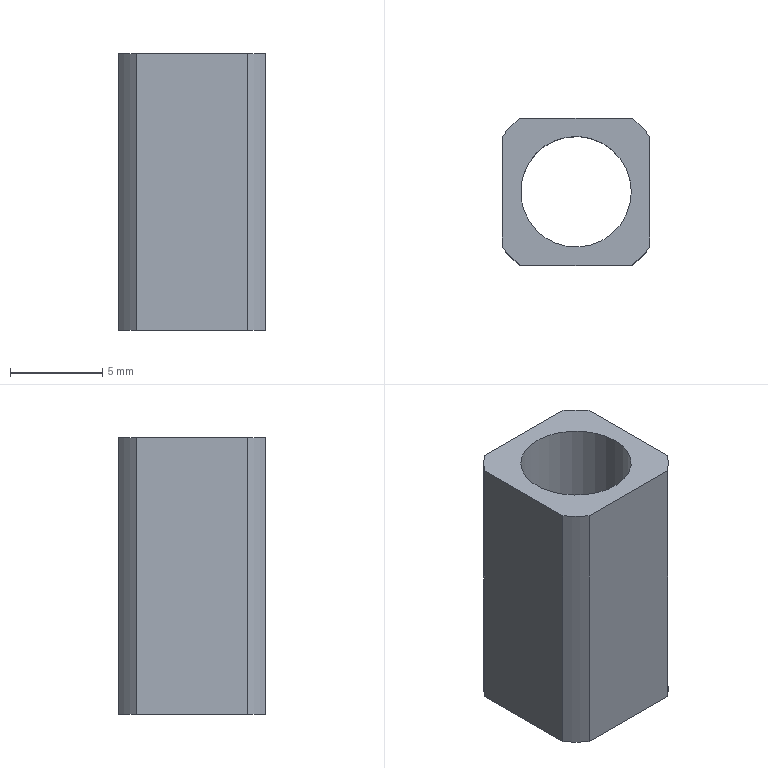Part | NX | 1 solid | 13 faces | box 8 x 8 x 15 mm | volume 464.552 mm3 | plane 7 | cylinder 6 | commonest cylinder face diameters 10 x4 6 x1 6.5 x1
STEP:
#1=CARTESIAN_POINT('',(3.,4.,15.));
#2=VERTEX_POINT('',#1);
#3=CARTESIAN_POINT('',(4.,3.,15.));
#4=VERTEX_POINT('',#3);
#5=CARTESIAN_POINT('',(0.,0.,15.));
#6=DIRECTION('',(0.,0.,-1.));
#7=DIRECTION('',(1.,0.,0.));
#8=AXIS2_PLACEMENT_3D('',#5,#6,#7);
#9=CIRCLE('',#8,5.);
#10=EDGE_CURVE('',#2,#4,#9,.T.);
#11=ORIENTED_EDGE('',*,*,#10,.T.);
#12=CARTESIAN_POINT('',(4.,3.,0.));
#13=VERTEX_POINT('',#12);
#14=CARTESIAN_POINT('',(4.,3.,0.));
#15=DIRECTION('',(0.,0.,1.));
#16=VECTOR('',#15,1000.);
#17=LINE('',#14,#16);
#18=EDGE_CURVE('',#13,#4,#17,.T.);
#19=ORIENTED_EDGE('',*,*,#18,.F.);
#20=CARTESIAN_POINT('',(3.,4.,0.));
#21=VERTEX_POINT('',#20);
#22=CARTESIAN_POINT('',(0.,0.,0.));
#23=DIRECTION('',(0.,0.,1.));
#24=DIRECTION('',(1.,0.,0.));
#25=AXIS2_PLACEMENT_3D('',#22,#23,#24);
#26=CIRCLE('',#25,5.);
#27=EDGE_CURVE('',#13,#21,#26,.T.);
#28=ORIENTED_EDGE('',*,*,#27,.T.);
#29=CARTESIAN_POINT('',(3.,4.,0.));
#30=DIRECTION('',(0.,0.,1.));
#31=VECTOR('',#30,1000.);
#32=LINE('',#29,#31);
#33=EDGE_CURVE('',#21,#2,#32,.T.);
#34=ORIENTED_EDGE('',*,*,#33,.T.);
#35=EDGE_LOOP('',(#11,#19,#28,#34));
#36=FACE_BOUND('',#35,.T.);
#37=CARTESIAN_POINT('',(0.,0.,0.));
#38=DIRECTION('',(0.,0.,1.));
#39=DIRECTION('',(1.,0.,0.));
#40=AXIS2_PLACEMENT_3D('',#37,#38,#39);
#41=CYLINDRICAL_SURFACE('',#40,5.);
#42=ADVANCED_FACE('',(#36),#41,.T.);
#43=CARTESIAN_POINT('',(-3.,4.,0.));
#44=VERTEX_POINT('',#43);
#45=CARTESIAN_POINT('',(-4.,3.,0.));
#46=VERTEX_POINT('',#45);
#47=CARTESIAN_POINT('',(0.,0.,0.));
#48=DIRECTION('',(0.,0.,1.));
#49=DIRECTION('',(1.,0.,0.));
#50=AXIS2_PLACEMENT_3D('',#47,#48,#49);
#51=CIRCLE('',#50,5.);
#52=EDGE_CURVE('',#44,#46,#51,.T.);
#53=ORIENTED_EDGE('',*,*,#52,.T.);
#54=CARTESIAN_POINT('',(-4.,3.,15.));
#55=VERTEX_POINT('',#54);
#56=CARTESIAN_POINT('',(-4.,3.,0.));
#57=DIRECTION('',(0.,0.,1.));
#58=VECTOR('',#57,1000.);
#59=LINE('',#56,#58);
#60=EDGE_CURVE('',#46,#55,#59,.T.);
#61=ORIENTED_EDGE('',*,*,#60,.T.);
#62=CARTESIAN_POINT('',(-3.,4.,15.));
#63=VERTEX_POINT('',#62);
#64=CARTESIAN_POINT('',(0.,0.,15.));
#65=DIRECTION('',(0.,0.,-1.));
#66=DIRECTION('',(1.,0.,0.));
#67=AXIS2_PLACEMENT_3D('',#64,#65,#66);
#68=CIRCLE('',#67,5.);
#69=EDGE_CURVE('',#55,#63,#68,.T.);
#70=ORIENTED_EDGE('',*,*,#69,.T.);
#71=CARTESIAN_POINT('',(-3.,4.,0.));
#72=DIRECTION('',(0.,0.,1.));
#73=VECTOR('',#72,1000.);
#74=LINE('',#71,#73);
#75=EDGE_CURVE('',#63,#44,#74,.F.);
#76=ORIENTED_EDGE('',*,*,#75,.T.);
#77=EDGE_LOOP('',(#53,#61,#70,#76));
#78=FACE_BOUND('',#77,.T.);
#79=CARTESIAN_POINT('',(0.,0.,0.));
#80=DIRECTION('',(0.,0.,1.));
#81=DIRECTION('',(1.,0.,0.));
#82=AXIS2_PLACEMENT_3D('',#79,#80,#81);
#83=CYLINDRICAL_SURFACE('',#82,5.);
#84=ADVANCED_FACE('',(#78),#83,.T.);
#85=CARTESIAN_POINT('',(-4.,-3.,0.));
#86=VERTEX_POINT('',#85);
#87=CARTESIAN_POINT('',(-3.,-4.,0.));
#88=VERTEX_POINT('',#87);
#89=CARTESIAN_POINT('',(0.,0.,0.));
#90=DIRECTION('',(0.,0.,1.));
#91=DIRECTION('',(1.,0.,0.));
#92=AXIS2_PLACEMENT_3D('',#89,#90,#91);
#93=CIRCLE('',#92,5.);
#94=EDGE_CURVE('',#86,#88,#93,.T.);
#95=ORIENTED_EDGE('',*,*,#94,.T.);
#96=CARTESIAN_POINT('',(-3.,-4.,15.));
#97=VERTEX_POINT('',#96);
#98=CARTESIAN_POINT('',(-3.,-4.,0.));
#99=DIRECTION('',(0.,0.,1.));
#100=VECTOR('',#99,1000.);
#101=LINE('',#98,#100);
#102=EDGE_CURVE('',#97,#88,#101,.F.);
#103=ORIENTED_EDGE('',*,*,#102,.F.);
#104=CARTESIAN_POINT('',(-4.,-3.,15.));
#105=VERTEX_POINT('',#104);
#106=CARTESIAN_POINT('',(0.,0.,15.));
#107=DIRECTION('',(0.,0.,-1.));
#108=DIRECTION('',(1.,0.,0.));
#109=AXIS2_PLACEMENT_3D('',#106,#107,#108);
#110=CIRCLE('',#109,5.);
#111=EDGE_CURVE('',#97,#105,#110,.T.);
#112=ORIENTED_EDGE('',*,*,#111,.T.);
#113=CARTESIAN_POINT('',(-4.,-3.,0.));
#114=DIRECTION('',(0.,0.,1.));
#115=VECTOR('',#114,1000.);
#116=LINE('',#113,#115);
#117=EDGE_CURVE('',#105,#86,#116,.F.);
#118=ORIENTED_EDGE('',*,*,#117,.T.);
#119=EDGE_LOOP('',(#95,#103,#112,#118));
#120=FACE_BOUND('',#119,.T.);
#121=CARTESIAN_POINT('',(0.,0.,0.));
#122=DIRECTION('',(0.,0.,1.));
#123=DIRECTION('',(1.,0.,0.));
#124=AXIS2_PLACEMENT_3D('',#121,#122,#123);
#125=CYLINDRICAL_SURFACE('',#124,5.);
#126=ADVANCED_FACE('',(#120),#125,.T.);
#127=CARTESIAN_POINT('',(4.,-3.,15.));
#128=VERTEX_POINT('',#127);
#129=CARTESIAN_POINT('',(3.,-4.,15.));
#130=VERTEX_POINT('',#129);
#131=CARTESIAN_POINT('',(0.,0.,15.));
#132=DIRECTION('',(0.,0.,-1.));
#133=DIRECTION('',(1.,0.,0.));
#134=AXIS2_PLACEMENT_3D('',#131,#132,#133);
#135=CIRCLE('',#134,5.);
#136=EDGE_CURVE('',#128,#130,#135,.T.);
#137=ORIENTED_EDGE('',*,*,#136,.T.);
#138=CARTESIAN_POINT('',(3.,-4.,0.));
#139=VERTEX_POINT('',#138);
#140=CARTESIAN_POINT('',(3.,-4.,0.));
#141=DIRECTION('',(0.,0.,1.));
#142=VECTOR('',#141,1000.);
#143=LINE('',#140,#142);
#144=EDGE_CURVE('',#139,#130,#143,.T.);
#145=ORIENTED_EDGE('',*,*,#144,.F.);
#146=CARTESIAN_POINT('',(4.,-3.,0.));
#147=VERTEX_POINT('',#146);
#148=CARTESIAN_POINT('',(0.,0.,0.));
#149=DIRECTION('',(0.,0.,1.));
#150=DIRECTION('',(1.,0.,0.));
#151=AXIS2_PLACEMENT_3D('',#148,#149,#150);
#152=CIRCLE('',#151,5.);
#153=EDGE_CURVE('',#139,#147,#152,.T.);
#154=ORIENTED_EDGE('',*,*,#153,.T.);
#155=CARTESIAN_POINT('',(4.,-3.,0.));
#156=DIRECTION('',(0.,0.,1.));
#157=VECTOR('',#156,1000.);
#158=LINE('',#155,#157);
#159=EDGE_CURVE('',#128,#147,#158,.F.);
#160=ORIENTED_EDGE('',*,*,#159,.F.);
#161=EDGE_LOOP('',(#137,#145,#154,#160));
#162=FACE_BOUND('',#161,.T.);
#163=CARTESIAN_POINT('',(0.,0.,0.));
#164=DIRECTION('',(0.,0.,1.));
#165=DIRECTION('',(1.,0.,0.));
#166=AXIS2_PLACEMENT_3D('',#163,#164,#165);
#167=CYLINDRICAL_SURFACE('',#166,5.);
#168=ADVANCED_FACE('',(#162),#167,.T.);
#169=CARTESIAN_POINT('',(3.25,0.,0.));
#170=VERTEX_POINT('',#169);
#171=CARTESIAN_POINT('',(0.,0.,0.));
#172=DIRECTION('',(0.,0.,1.));
#173=DIRECTION('',(1.,0.,0.));
#174=AXIS2_PLACEMENT_3D('',#171,#172,#173);
#175=CIRCLE('',#174,3.25);
#176=EDGE_CURVE('',#170,#170,#175,.T.);
#177=ORIENTED_EDGE('',*,*,#176,.T.);
#178=EDGE_LOOP('',(#177));
#179=FACE_BOUND('',#178,.T.);
#180=CARTESIAN_POINT('',(4.,0.,0.));
#181=DIRECTION('',(0.,1.,0.));
#182=VECTOR('',#181,1000.);
#183=LINE('',#180,#182);
#184=EDGE_CURVE('',#13,#147,#183,.F.);
#185=ORIENTED_EDGE('',*,*,#184,.T.);
#186=ORIENTED_EDGE('',*,*,#153,.F.);
#187=CARTESIAN_POINT('',(0.,-4.,0.));
#188=DIRECTION('',(1.,0.,0.));
#189=VECTOR('',#188,1000.);
#190=LINE('',#187,#189);
#191=EDGE_CURVE('',#139,#88,#190,.F.);
#192=ORIENTED_EDGE('',*,*,#191,.T.);
#193=ORIENTED_EDGE('',*,*,#94,.F.);
#194=CARTESIAN_POINT('',(-4.,0.,0.));
#195=DIRECTION('',(0.,-1.,0.));
#196=VECTOR('',#195,1000.);
#197=LINE('',#194,#196);
#198=EDGE_CURVE('',#46,#86,#197,.T.);
#199=ORIENTED_EDGE('',*,*,#198,.F.);
#200=ORIENTED_EDGE('',*,*,#52,.F.);
#201=CARTESIAN_POINT('',(0.,4.,0.));
#202=DIRECTION('',(-1.,0.,0.));
#203=VECTOR('',#202,1000.);
#204=LINE('',#201,#203);
#205=EDGE_CURVE('',#44,#21,#204,.F.);
#206=ORIENTED_EDGE('',*,*,#205,.T.);
#207=ORIENTED_EDGE('',*,*,#27,.F.);
#208=EDGE_LOOP('',(#185,#186,#192,#193,#199,#200,#206,#207));
#209=FACE_BOUND('',#208,.T.);
#210=CARTESIAN_POINT('',(0.,0.,0.));
#211=DIRECTION('',(0.,0.,-1.));
#212=DIRECTION('',(-1.,0.,0.));
#213=AXIS2_PLACEMENT_3D('',#210,#211,#212);
#214=PLANE('',#213);
#215=ADVANCED_FACE('',(#179,#209),#214,.T.);
#216=CARTESIAN_POINT('',(3.,0.,15.));
#217=VERTEX_POINT('',#216);
#218=CARTESIAN_POINT('',(0.,0.,15.));
#219=DIRECTION('',(0.,0.,-1.));
#220=DIRECTION('',(1.,0.,0.));
#221=AXIS2_PLACEMENT_3D('',#218,#219,#220);
#222=CIRCLE('',#221,3.);
#223=EDGE_CURVE('',#217,#217,#222,.T.);
#224=ORIENTED_EDGE('',*,*,#223,.T.);
#225=EDGE_LOOP('',(#224));
#226=FACE_BOUND('',#225,.T.);
#227=CARTESIAN_POINT('',(0.,-4.,15.));
#228=DIRECTION('',(-1.,0.,0.));
#229=VECTOR('',#228,1000.);
#230=LINE('',#227,#229);
#231=EDGE_CURVE('',#130,#97,#230,.T.);
#232=ORIENTED_EDGE('',*,*,#231,.F.);
#233=ORIENTED_EDGE('',*,*,#136,.F.);
#234=CARTESIAN_POINT('',(4.,0.,15.));
#235=DIRECTION('',(0.,-1.,0.));
#236=VECTOR('',#235,1000.);
#237=LINE('',#234,#236);
#238=EDGE_CURVE('',#4,#128,#237,.T.);
#239=ORIENTED_EDGE('',*,*,#238,.F.);
#240=ORIENTED_EDGE('',*,*,#10,.F.);
#241=CARTESIAN_POINT('',(0.,4.,15.));
#242=DIRECTION('',(1.,0.,0.));
#243=VECTOR('',#242,1000.);
#244=LINE('',#241,#243);
#245=EDGE_CURVE('',#63,#2,#244,.T.);
#246=ORIENTED_EDGE('',*,*,#245,.F.);
#247=ORIENTED_EDGE('',*,*,#69,.F.);
#248=CARTESIAN_POINT('',(-4.,0.,15.));
#249=DIRECTION('',(0.,1.,0.));
#250=VECTOR('',#249,1000.);
#251=LINE('',#248,#250);
#252=EDGE_CURVE('',#105,#55,#251,.T.);
#253=ORIENTED_EDGE('',*,*,#252,.F.);
#254=ORIENTED_EDGE('',*,*,#111,.F.);
#255=EDGE_LOOP('',(#232,#233,#239,#240,#246,#247,#253,#254));
#256=FACE_BOUND('',#255,.T.);
#257=CARTESIAN_POINT('',(0.,0.,15.));
#258=DIRECTION('',(0.,0.,1.));
#259=DIRECTION('',(1.,0.,0.));
#260=AXIS2_PLACEMENT_3D('',#257,#258,#259);
#261=PLANE('',#260);
#262=ADVANCED_FACE('',(#226,#256),#261,.T.);
#263=ORIENTED_EDGE('',*,*,#75,.F.);
#264=ORIENTED_EDGE('',*,*,#245,.T.);
#265=ORIENTED_EDGE('',*,*,#33,.F.);
#266=ORIENTED_EDGE('',*,*,#205,.F.);
#267=EDGE_LOOP('',(#263,#264,#265,#266));
#268=FACE_BOUND('',#267,.T.);
#269=CARTESIAN_POINT('',(0.,4.,0.));
#270=DIRECTION('',(0.,1.,0.));
#271=DIRECTION('',(0.,0.,1.));
#272=AXIS2_PLACEMENT_3D('',#269,#270,#271);
#273=PLANE('',#272);
#274=ADVANCED_FACE('',(#268),#273,.T.);
#275=ORIENTED_EDGE('',*,*,#117,.F.);
#276=ORIENTED_EDGE('',*,*,#252,.T.);
#277=ORIENTED_EDGE('',*,*,#60,.F.);
#278=ORIENTED_EDGE('',*,*,#198,.T.);
#279=EDGE_LOOP('',(#275,#276,#277,#278));
#280=FACE_BOUND('',#279,.T.);
#281=CARTESIAN_POINT('',(-4.,0.,0.));
#282=DIRECTION('',(-1.,0.,0.));
#283=DIRECTION('',(0.,0.,1.));
#284=AXIS2_PLACEMENT_3D('',#281,#282,#283);
#285=PLANE('',#284);
#286=ADVANCED_FACE('',(#280),#285,.T.);
#287=ORIENTED_EDGE('',*,*,#18,.T.);
#288=ORIENTED_EDGE('',*,*,#238,.T.);
#289=ORIENTED_EDGE('',*,*,#159,.T.);
#290=ORIENTED_EDGE('',*,*,#184,.F.);
#291=EDGE_LOOP('',(#287,#288,#289,#290));
#292=FACE_BOUND('',#291,.T.);
#293=CARTESIAN_POINT('',(4.,0.,0.));
#294=DIRECTION('',(1.,0.,0.));
#295=DIRECTION('',(0.,0.,-1.));
#296=AXIS2_PLACEMENT_3D('',#293,#294,#295);
#297=PLANE('',#296);
#298=ADVANCED_FACE('',(#292),#297,.T.);
#299=ORIENTED_EDGE('',*,*,#144,.T.);
#300=ORIENTED_EDGE('',*,*,#231,.T.);
#301=ORIENTED_EDGE('',*,*,#102,.T.);
#302=ORIENTED_EDGE('',*,*,#191,.F.);
#303=EDGE_LOOP('',(#299,#300,#301,#302));
#304=FACE_BOUND('',#303,.T.);
#305=CARTESIAN_POINT('',(0.,-4.,0.));
#306=DIRECTION('',(0.,-1.,0.));
#307=DIRECTION('',(0.,0.,-1.));
#308=AXIS2_PLACEMENT_3D('',#305,#306,#307);
#309=PLANE('',#308);
#310=ADVANCED_FACE('',(#304),#309,.T.);
#311=CARTESIAN_POINT('',(3.,0.,9.));
#312=VERTEX_POINT('',#311);
#313=CARTESIAN_POINT('',(0.,0.,9.));
#314=DIRECTION('',(0.,0.,1.));
#315=DIRECTION('',(1.,0.,0.));
#316=AXIS2_PLACEMENT_3D('',#313,#314,#315);
#317=CIRCLE('',#316,3.);
#318=EDGE_CURVE('',#312,#312,#317,.T.);
#319=ORIENTED_EDGE('',*,*,#318,.T.);
#320=EDGE_LOOP('',(#319));
#321=FACE_BOUND('',#320,.T.);
#322=CARTESIAN_POINT('',(3.25,0.,9.));
#323=VERTEX_POINT('',#322);
#324=CARTESIAN_POINT('',(0.,0.,9.));
#325=DIRECTION('',(0.,0.,-1.));
#326=DIRECTION('',(1.,0.,0.));
#327=AXIS2_PLACEMENT_3D('',#324,#325,#326);
#328=CIRCLE('',#327,3.25);
#329=EDGE_CURVE('',#323,#323,#328,.F.);
#330=ORIENTED_EDGE('',*,*,#329,.F.);
#331=EDGE_LOOP('',(#330));
#332=FACE_BOUND('',#331,.T.);
#333=CARTESIAN_POINT('',(0.,0.,9.));
#334=DIRECTION('',(0.,0.,1.));
#335=DIRECTION('',(1.,0.,0.));
#336=AXIS2_PLACEMENT_3D('',#333,#334,#335);
#337=PLANE('',#336);
#338=ADVANCED_FACE('',(#321,#332),#337,.F.);
#339=ORIENTED_EDGE('',*,*,#329,.T.);
#340=EDGE_LOOP('',(#339));
#341=FACE_BOUND('',#340,.T.);
#342=ORIENTED_EDGE('',*,*,#176,.F.);
#343=EDGE_LOOP('',(#342));
#344=FACE_BOUND('',#343,.T.);
#345=CARTESIAN_POINT('',(0.,0.,0.));
#346=DIRECTION('',(0.,0.,1.));
#347=DIRECTION('',(1.,0.,0.));
#348=AXIS2_PLACEMENT_3D('',#345,#346,#347);
#349=CYLINDRICAL_SURFACE('',#348,3.25);
#350=ADVANCED_FACE('',(#341,#344),#349,.F.);
#351=ORIENTED_EDGE('',*,*,#223,.F.);
#352=EDGE_LOOP('',(#351));
#353=FACE_BOUND('',#352,.T.);
#354=ORIENTED_EDGE('',*,*,#318,.F.);
#355=EDGE_LOOP('',(#354));
#356=FACE_BOUND('',#355,.T.);
#357=CARTESIAN_POINT('',(0.,0.,0.));
#358=DIRECTION('',(0.,0.,1.));
#359=DIRECTION('',(1.,0.,0.));
#360=AXIS2_PLACEMENT_3D('',#357,#358,#359);
#361=CYLINDRICAL_SURFACE('',#360,3.);
#362=ADVANCED_FACE('',(#353,#356),#361,.F.);
#363=CLOSED_SHELL('',(#42,#84,#126,#168,#215,#262,#274,#286,#298,#310,#338,#350,#362));
#364=MANIFOLD_SOLID_BREP('',#363);
#365=(LENGTH_UNIT()NAMED_UNIT(*)SI_UNIT(.MILLI.,.METRE.));
#366=UNCERTAINTY_MEASURE_WITH_UNIT(LENGTH_MEASURE(0.00001),#365,'','');
#367=(NAMED_UNIT(*)PLANE_ANGLE_UNIT()SI_UNIT($,.RADIAN.));
#368=(NAMED_UNIT(*)SI_UNIT($,.STERADIAN.)SOLID_ANGLE_UNIT());
#369=(GEOMETRIC_REPRESENTATION_CONTEXT(3)GLOBAL_UNCERTAINTY_ASSIGNED_CONTEXT((#366))GLOBAL_UNIT_ASSIGNED_CONTEXT((#365,#367,#368))REPRESENTATION_CONTEXT('',''));
#370=ADVANCED_BREP_SHAPE_REPRESENTATION('',(#364),#369);